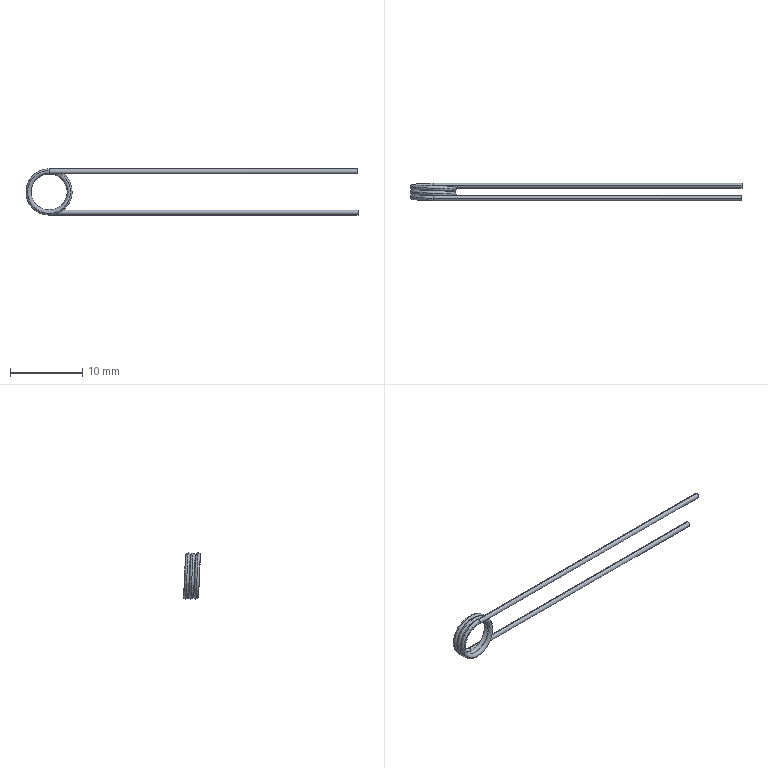Part | SolidWorks | features CompositeCurve 1, Helix 1, MoveFace 1, Sweep 1 | 1 solid | 9 faces | box 46.05 x 2.45 x 6.4 mm | volume 49.652 mm3 | cylinder 4 | spline 3 | plane 2 | commonest cylinder face diameters 0.7 x4
STEP:
#1=CARTESIAN_POINT('',(42.85,1.75,-3.2));
#2=VERTEX_POINT('',#1);
#3=CARTESIAN_POINT('',(42.85,1.75,-2.5));
#4=VERTEX_POINT('',#3);
#5=CARTESIAN_POINT('',(42.85,1.75,-2.85));
#6=DIRECTION('',(1.,0.,0.));
#7=DIRECTION('',(0.,0.00009155,-1.));
#8=AXIS2_PLACEMENT_3D('',#5,#6,#7);
#9=CIRCLE('',#8,0.35);
#10=EDGE_CURVE('',#2,#4,#9,.T.);
#11=ORIENTED_EDGE('',*,*,#10,.F.);
#12=CARTESIAN_POINT('',(-0.000000536,1.75,-3.2));
#13=VERTEX_POINT('',#12);
#14=CARTESIAN_POINT('',(12.85,1.75,-3.2));
#15=DIRECTION('',(-1.,0.,0.));
#16=VECTOR('',#15,1000.);
#17=LINE('',#14,#16);
#18=EDGE_CURVE('',#2,#13,#17,.T.);
#19=ORIENTED_EDGE('',*,*,#18,.T.);
#20=CARTESIAN_POINT('',(-0.006305,2.074,-2.979));
#21=VERTEX_POINT('',#20);
#22=CARTESIAN_POINT('',(0.,1.75,-2.85));
#23=DIRECTION('',(1.,0.,0.));
#24=DIRECTION('',(0.,0.00009155,-1.));
#25=AXIS2_PLACEMENT_3D('',#22,#23,#24);
#26=CIRCLE('',#25,0.35);
#27=EDGE_CURVE('',#13,#21,#26,.T.);
#28=ORIENTED_EDGE('',*,*,#27,.T.);
#29=CARTESIAN_POINT('',(0.,1.75,-2.5));
#30=VERTEX_POINT('',#29);
#31=CARTESIAN_POINT('',(0.,1.75,-2.85));
#32=DIRECTION('',(1.,0.,0.));
#33=DIRECTION('',(0.,0.00009155,-1.));
#34=AXIS2_PLACEMENT_3D('',#31,#32,#33);
#35=CIRCLE('',#34,0.35);
#36=EDGE_CURVE('',#21,#30,#35,.T.);
#37=ORIENTED_EDGE('',*,*,#36,.T.);
#38=CARTESIAN_POINT('',(12.85,1.75,-2.5));
#39=DIRECTION('',(-1.,0.,0.));
#40=VECTOR('',#39,1000.);
#41=LINE('',#38,#40);
#42=EDGE_CURVE('',#4,#30,#41,.T.);
#43=ORIENTED_EDGE('',*,*,#42,.F.);
#44=EDGE_LOOP('',(#11,#19,#28,#37,#43));
#45=FACE_OUTER_BOUND('',#44,.T.);
#46=CARTESIAN_POINT('',(12.85,1.75,-2.85));
#47=DIRECTION('',(-1.,0.,0.));
#48=DIRECTION('',(0.,0.,1.));
#49=AXIS2_PLACEMENT_3D('',#46,#47,#48);
#50=CYLINDRICAL_SURFACE('',#49,0.35);
#51=ADVANCED_FACE('',(#45),#50,.T.);
#52=CARTESIAN_POINT('',(0.006305,0.3239,2.979));
#53=VERTEX_POINT('',#52);
#54=CARTESIAN_POINT('',(0.,0.,3.2));
#55=VERTEX_POINT('',#54);
#56=CARTESIAN_POINT('',(0.006305,0.3239,2.979));
#57=CARTESIAN_POINT('',(0.01048,0.2681,3.104));
#58=CARTESIAN_POINT('',(0.005425,0.1388,3.2));
#59=CARTESIAN_POINT('',(0.,0.,3.2));
#60=B_SPLINE_CURVE_WITH_KNOTS('',3,(#56,#57,#58,#59),.UNSPECIFIED.,.F.,.F.,(4,4),(0.00002721,0.1895),.UNSPECIFIED.);
#61=EDGE_CURVE('',#53,#55,#60,.T.);
#62=ORIENTED_EDGE('',*,*,#61,.T.);
#63=CARTESIAN_POINT('',(42.85,0.,3.2));
#64=VERTEX_POINT('',#63);
#65=CARTESIAN_POINT('',(0.,0.,3.2));
#66=DIRECTION('',(1.,0.,0.));
#67=VECTOR('',#66,1000.);
#68=LINE('',#65,#67);
#69=EDGE_CURVE('',#55,#64,#68,.T.);
#70=ORIENTED_EDGE('',*,*,#69,.T.);
#71=CARTESIAN_POINT('',(42.85,0.,2.5));
#72=VERTEX_POINT('',#71);
#73=CARTESIAN_POINT('',(42.85,0.,2.85));
#74=DIRECTION('',(-1.,0.,0.));
#75=DIRECTION('',(0.,0.,1.));
#76=AXIS2_PLACEMENT_3D('',#73,#74,#75);
#77=CIRCLE('',#76,0.35);
#78=EDGE_CURVE('',#64,#72,#77,.T.);
#79=ORIENTED_EDGE('',*,*,#78,.T.);
#80=CARTESIAN_POINT('',(0.,0.,2.5));
#81=VERTEX_POINT('',#80);
#82=CARTESIAN_POINT('',(0.,0.,2.5));
#83=DIRECTION('',(1.,0.,0.));
#84=VECTOR('',#83,1000.);
#85=LINE('',#82,#84);
#86=EDGE_CURVE('',#81,#72,#85,.T.);
#87=ORIENTED_EDGE('',*,*,#86,.F.);
#88=CARTESIAN_POINT('',(0.,0.,2.85));
#89=DIRECTION('',(-1.,0.,0.));
#90=DIRECTION('',(0.,0.,1.));
#91=AXIS2_PLACEMENT_3D('',#88,#89,#90);
#92=CIRCLE('',#91,0.35);
#93=EDGE_CURVE('',#53,#81,#92,.T.);
#94=ORIENTED_EDGE('',*,*,#93,.F.);
#95=EDGE_LOOP('',(#62,#70,#79,#87,#94));
#96=FACE_OUTER_BOUND('',#95,.T.);
#97=CARTESIAN_POINT('',(0.,0.,2.85));
#98=DIRECTION('',(1.,0.,0.));
#99=DIRECTION('',(0.,0.,-1.));
#100=AXIS2_PLACEMENT_3D('',#97,#98,#99);
#101=CYLINDRICAL_SURFACE('',#100,0.35);
#102=ADVANCED_FACE('',(#96),#101,.T.);
#103=ORIENTED_EDGE('',*,*,#18,.F.);
#104=CARTESIAN_POINT('',(42.85,1.75,-2.85));
#105=DIRECTION('',(1.,0.,0.));
#106=DIRECTION('',(0.,0.00009155,-1.));
#107=AXIS2_PLACEMENT_3D('',#104,#105,#106);
#108=CIRCLE('',#107,0.35);
#109=EDGE_CURVE('',#4,#2,#108,.T.);
#110=ORIENTED_EDGE('',*,*,#109,.F.);
#111=ORIENTED_EDGE('',*,*,#42,.T.);
#112=CARTESIAN_POINT('',(0.006304,1.426,-2.979));
#113=VERTEX_POINT('',#112);
#114=CARTESIAN_POINT('',(0.,1.75,-2.85));
#115=DIRECTION('',(1.,0.,0.));
#116=DIRECTION('',(0.,0.00009155,-1.));
#117=AXIS2_PLACEMENT_3D('',#114,#115,#116);
#118=CIRCLE('',#117,0.35);
#119=EDGE_CURVE('',#30,#113,#118,.T.);
#120=ORIENTED_EDGE('',*,*,#119,.T.);
#121=CARTESIAN_POINT('',(0.,1.75,-2.85));
#122=DIRECTION('',(1.,0.,0.));
#123=DIRECTION('',(0.,0.00009155,-1.));
#124=AXIS2_PLACEMENT_3D('',#121,#122,#123);
#125=CIRCLE('',#124,0.35);
#126=EDGE_CURVE('',#113,#13,#125,.T.);
#127=ORIENTED_EDGE('',*,*,#126,.T.);
#128=EDGE_LOOP('',(#103,#110,#111,#120,#127));
#129=FACE_OUTER_BOUND('',#128,.T.);
#130=CARTESIAN_POINT('',(12.85,1.75,-2.85));
#131=DIRECTION('',(-1.,0.,0.));
#132=DIRECTION('',(0.,0.,1.));
#133=AXIS2_PLACEMENT_3D('',#130,#131,#132);
#134=CYLINDRICAL_SURFACE('',#133,0.35);
#135=ADVANCED_FACE('',(#129),#134,.T.);
#136=ORIENTED_EDGE('',*,*,#36,.F.);
#137=CARTESIAN_POINT('',(0.006305,0.3239,2.979));
#138=CARTESIAN_POINT('',(-0.7712,0.3519,2.981));
#139=CARTESIAN_POINT('',(-1.545,0.381,2.663));
#140=CARTESIAN_POINT('',(-2.649,0.4392,1.566));
#141=CARTESIAN_POINT('',(-2.975,0.4683,0.7939));
#142=CARTESIAN_POINT('',(-2.98,0.5195,-0.5733));
#143=CARTESIAN_POINT('',(-2.806,0.5413,-1.156));
#144=CARTESIAN_POINT('',(-2.162,0.585,-2.13));
#145=CARTESIAN_POINT('',(-1.69,0.6069,-2.521));
#146=CARTESIAN_POINT('',(-0.4324,0.658,-3.048));
#147=CARTESIAN_POINT('',(0.405,0.6871,-3.052));
#148=CARTESIAN_POINT('',(1.67,0.7383,-2.534));
#149=CARTESIAN_POINT('',(2.142,0.7601,-2.15));
#150=CARTESIAN_POINT('',(2.795,0.8037,-1.182));
#151=CARTESIAN_POINT('',(2.976,0.8257,-0.5972));
#152=CARTESIAN_POINT('',(2.981,0.8768,0.7668));
#153=CARTESIAN_POINT('',(2.665,0.9058,1.542));
#154=CARTESIAN_POINT('',(1.702,0.957,2.513));
#155=CARTESIAN_POINT('',(1.167,0.9788,2.801));
#156=CARTESIAN_POINT('',(0.02248,1.022,3.035));
#157=CARTESIAN_POINT('',(-0.587,1.044,2.978));
#158=CARTESIAN_POINT('',(-1.849,1.096,2.461));
#159=CARTESIAN_POINT('',(-2.445,1.125,1.872));
#160=CARTESIAN_POINT('',(-2.973,1.176,0.6109));
#161=CARTESIAN_POINT('',(-3.035,1.198,0.005944));
#162=CARTESIAN_POINT('',(-2.812,1.241,-1.14));
#163=CARTESIAN_POINT('',(-2.526,1.263,-1.682));
#164=CARTESIAN_POINT('',(-1.566,1.314,-2.65));
#165=CARTESIAN_POINT('',(-0.7938,1.343,-2.975));
#166=CARTESIAN_POINT('',(0.5733,1.395,-2.98));
#167=CARTESIAN_POINT('',(1.156,1.416,-2.806));
#168=CARTESIAN_POINT('',(2.13,1.46,-2.162));
#169=CARTESIAN_POINT('',(2.521,1.482,-1.69));
#170=CARTESIAN_POINT('',(3.048,1.533,-0.4324));
#171=CARTESIAN_POINT('',(3.052,1.562,0.405));
#172=CARTESIAN_POINT('',(2.534,1.613,1.67));
#173=CARTESIAN_POINT('',(2.15,1.635,2.142));
#174=CARTESIAN_POINT('',(1.182,1.679,2.795));
#175=CARTESIAN_POINT('',(0.5972,1.701,2.976));
#176=CARTESIAN_POINT('',(-0.7668,1.752,2.981));
#177=CARTESIAN_POINT('',(-1.542,1.781,2.665));
#178=CARTESIAN_POINT('',(-2.513,1.832,1.702));
#179=CARTESIAN_POINT('',(-2.801,1.854,1.167));
#180=CARTESIAN_POINT('',(-3.034,1.897,0.0225));
#181=CARTESIAN_POINT('',(-2.978,1.919,-0.587));
#182=CARTESIAN_POINT('',(-2.46,1.971,-1.85));
#183=CARTESIAN_POINT('',(-1.872,2.,-2.445));
#184=CARTESIAN_POINT('',(-0.7917,2.043,-2.897));
#185=CARTESIAN_POINT('',(-0.4042,2.058,-2.976));
#186=CARTESIAN_POINT('',(-0.006305,2.074,-2.979));
#187=B_SPLINE_CURVE_WITH_KNOTS('',3,(#137,#138,#139,#140,#141,#142,#143,#144,#145,#146,#147,#148,#149,#150,#151,#152,#153,#154,#155,#156,#157,#158,#159,#160,#161,#162,#163,#164,#165,#166,#167,#168,#169,#170,#171,#172,#173,#174,#175,#176,#177,#178,#179,#180,#181,#182,#183,#184,#185,#186),.UNSPECIFIED.,.F.,.F.,(4,2,2,2,2,2,2,2,2,2,2,2,2,2,2,2,2,2,2,2,2,2,2,2,4),(0.,0.04998,0.09999,0.1375,0.175,0.225,0.2625,0.3,0.35,0.3875,0.425,0.475,0.5125,0.55,0.6,0.6375,0.675,0.725,0.7625,0.8,0.85,0.8875,0.925,0.975,1.),.UNSPECIFIED.);
#188=EDGE_CURVE('',#53,#21,#187,.T.);
#189=ORIENTED_EDGE('',*,*,#188,.F.);
#190=ORIENTED_EDGE('',*,*,#93,.T.);
#191=CARTESIAN_POINT('',(-0.006304,-0.3239,2.979));
#192=VERTEX_POINT('',#191);
#193=CARTESIAN_POINT('',(0.,0.,2.85));
#194=DIRECTION('',(-1.,0.,0.));
#195=DIRECTION('',(0.,0.,1.));
#196=AXIS2_PLACEMENT_3D('',#193,#194,#195);
#197=CIRCLE('',#196,0.35);
#198=EDGE_CURVE('',#81,#192,#197,.T.);
#199=ORIENTED_EDGE('',*,*,#198,.T.);
#200=CARTESIAN_POINT('',(0.006304,1.426,-2.979));
#201=CARTESIAN_POINT('',(-0.379,1.413,-2.98));
#202=CARTESIAN_POINT('',(-0.7673,1.398,-2.904));
#203=CARTESIAN_POINT('',(-1.851,1.354,-2.461));
#204=CARTESIAN_POINT('',(-2.445,1.325,-1.871));
#205=CARTESIAN_POINT('',(-2.973,1.274,-0.6122));
#206=CARTESIAN_POINT('',(-3.035,1.252,-0.003211));
#207=CARTESIAN_POINT('',(-2.811,1.209,1.143));
#208=CARTESIAN_POINT('',(-2.527,1.187,1.681));
#209=CARTESIAN_POINT('',(-1.565,1.136,2.652));
#210=CARTESIAN_POINT('',(-0.792,1.107,2.975));
#211=CARTESIAN_POINT('',(0.572,1.056,2.981));
#212=CARTESIAN_POINT('',(1.158,1.034,2.805));
#213=CARTESIAN_POINT('',(2.132,0.99,2.16));
#214=CARTESIAN_POINT('',(2.52,0.9682,1.692));
#215=CARTESIAN_POINT('',(3.049,0.917,0.4308));
#216=CARTESIAN_POINT('',(3.052,0.8879,-0.4067));
#217=CARTESIAN_POINT('',(2.535,0.8368,-1.669));
#218=CARTESIAN_POINT('',(2.148,0.8149,-2.144));
#219=CARTESIAN_POINT('',(1.18,0.7712,-2.796));
#220=CARTESIAN_POINT('',(0.5985,0.7494,-2.976));
#221=CARTESIAN_POINT('',(-0.7686,0.6982,-2.981));
#222=CARTESIAN_POINT('',(-1.544,0.6692,-2.664));
#223=CARTESIAN_POINT('',(-2.512,0.6181,-1.703));
#224=CARTESIAN_POINT('',(-2.802,0.5961,-1.164));
#225=CARTESIAN_POINT('',(-3.035,0.5525,-0.01977));
#226=CARTESIAN_POINT('',(-2.978,0.5307,0.5858));
#227=CARTESIAN_POINT('',(-2.46,0.4795,1.851));
#228=CARTESIAN_POINT('',(-1.87,0.4504,2.445));
#229=CARTESIAN_POINT('',(-0.6122,0.3993,2.973));
#230=CARTESIAN_POINT('',(-0.003226,0.3774,3.035));
#231=CARTESIAN_POINT('',(1.143,0.3337,2.811));
#232=CARTESIAN_POINT('',(1.681,0.3119,2.527));
#233=CARTESIAN_POINT('',(2.652,0.2607,1.565));
#234=CARTESIAN_POINT('',(2.975,0.2317,0.792));
#235=CARTESIAN_POINT('',(2.981,0.1806,-0.572));
#236=CARTESIAN_POINT('',(2.805,0.1586,-1.158));
#237=CARTESIAN_POINT('',(2.16,0.115,-2.132));
#238=CARTESIAN_POINT('',(1.692,0.09317,-2.52));
#239=CARTESIAN_POINT('',(0.4308,0.04196,-3.049));
#240=CARTESIAN_POINT('',(-0.4067,0.01292,-3.052));
#241=CARTESIAN_POINT('',(-1.669,-0.03818,-2.535));
#242=CARTESIAN_POINT('',(-2.144,-0.06013,-2.148));
#243=CARTESIAN_POINT('',(-2.796,-0.1038,-1.18));
#244=CARTESIAN_POINT('',(-2.976,-0.1256,-0.5985));
#245=CARTESIAN_POINT('',(-2.981,-0.1768,0.7687));
#246=CARTESIAN_POINT('',(-2.663,-0.2059,1.544));
#247=CARTESIAN_POINT('',(-1.567,-0.2642,2.65));
#248=CARTESIAN_POINT('',(-0.7966,-0.2932,2.975));
#249=CARTESIAN_POINT('',(-0.006304,-0.3239,2.979));
#250=B_SPLINE_CURVE_WITH_KNOTS('',3,(#200,#201,#202,#203,#204,#205,#206,#207,#208,#209,#210,#211,#212,#213,#214,#215,#216,#217,#218,#219,#220,#221,#222,#223,#224,#225,#226,#227,#228,#229,#230,#231,#232,#233,#234,#235,#236,#237,#238,#239,#240,#241,#242,#243,#244,#245,#246,#247,#248,#249),.UNSPECIFIED.,.F.,.F.,(4,2,2,2,2,2,2,2,2,2,2,2,2,2,2,2,2,2,2,2,2,2,2,2,4),(0.,0.02496,0.07501,0.1125,0.15,0.2,0.2375,0.275,0.325,0.3625,0.4,0.45,0.4875,0.525,0.575,0.6125,0.65,0.7,0.7375,0.775,0.825,0.8625,0.9,0.95,1.),.UNSPECIFIED.);
#251=EDGE_CURVE('',#113,#192,#250,.T.);
#252=ORIENTED_EDGE('',*,*,#251,.F.);
#253=ORIENTED_EDGE('',*,*,#119,.F.);
#254=EDGE_LOOP('',(#136,#189,#190,#199,#252,#253));
#255=FACE_OUTER_BOUND('',#254,.T.);
#256=CARTESIAN_POINT('',(-0.01261,2.073,-2.978));
#257=CARTESIAN_POINT('',(-0.9931,2.036,-2.974));
#258=CARTESIAN_POINT('',(-1.942,2.,-2.452));
#259=CARTESIAN_POINT('',(-3.022,1.927,-0.8338));
#260=CARTESIAN_POINT('',(-3.123,1.89,0.2539));
#261=CARTESIAN_POINT('',(-2.369,1.817,2.048));
#262=CARTESIAN_POINT('',(-1.523,1.781,2.732));
#263=CARTESIAN_POINT('',(0.3864,1.708,3.111));
#264=CARTESIAN_POINT('',(1.43,1.671,2.788));
#265=CARTESIAN_POINT('',(2.798,1.599,1.405));
#266=CARTESIAN_POINT('',(3.107,1.562,0.3615));
#267=CARTESIAN_POINT('',(2.726,1.489,-1.547));
#268=CARTESIAN_POINT('',(2.029,1.453,-2.388));
#269=CARTESIAN_POINT('',(0.2273,1.38,-3.123));
#270=CARTESIAN_POINT('',(-0.8551,1.343,-3.009));
#271=CARTESIAN_POINT('',(-2.473,1.271,-1.927));
#272=CARTESIAN_POINT('',(-2.982,1.234,-0.9604));
#273=CARTESIAN_POINT('',(-2.972,1.161,0.9852));
#274=CARTESIAN_POINT('',(-2.453,1.125,1.942));
#275=CARTESIAN_POINT('',(-0.8335,1.052,3.022));
#276=CARTESIAN_POINT('',(0.2539,1.015,3.123));
#277=CARTESIAN_POINT('',(2.048,0.9425,2.369));
#278=CARTESIAN_POINT('',(2.732,0.9059,1.523));
#279=CARTESIAN_POINT('',(3.111,0.8331,-0.3864));
#280=CARTESIAN_POINT('',(2.788,0.7965,-1.43));
#281=CARTESIAN_POINT('',(1.405,0.7237,-2.798));
#282=CARTESIAN_POINT('',(0.3615,0.6872,-3.107));
#283=CARTESIAN_POINT('',(-1.547,0.6143,-2.726));
#284=CARTESIAN_POINT('',(-2.388,0.5777,-2.029));
#285=CARTESIAN_POINT('',(-3.123,0.505,-0.2273));
#286=CARTESIAN_POINT('',(-3.009,0.4684,0.8554));
#287=CARTESIAN_POINT('',(-1.927,0.3956,2.473));
#288=CARTESIAN_POINT('',(-0.9676,0.3593,2.982));
#289=CARTESIAN_POINT('',(0.01261,0.3226,2.978));
#290=CARTESIAN_POINT('',(-0.0161,2.162,-2.771));
#291=CARTESIAN_POINT('',(-0.9269,2.125,-2.766));
#292=CARTESIAN_POINT('',(-1.811,2.089,-2.279));
#293=CARTESIAN_POINT('',(-2.813,2.016,-0.7712));
#294=CARTESIAN_POINT('',(-2.906,1.979,0.2409));
#295=CARTESIAN_POINT('',(-2.201,1.907,1.909));
#296=CARTESIAN_POINT('',(-1.413,1.87,2.545));
#297=CARTESIAN_POINT('',(0.3644,1.797,2.894));
#298=CARTESIAN_POINT('',(1.334,1.761,2.592));
#299=CARTESIAN_POINT('',(2.606,1.688,1.303));
#300=CARTESIAN_POINT('',(2.892,1.651,0.3318));
#301=CARTESIAN_POINT('',(2.535,1.579,-1.444));
#302=CARTESIAN_POINT('',(1.884,1.542,-2.225));
#303=CARTESIAN_POINT('',(0.2064,1.469,-2.907));
#304=CARTESIAN_POINT('',(-0.8001,1.433,-2.799));
#305=CARTESIAN_POINT('',(-2.304,1.36,-1.789));
#306=CARTESIAN_POINT('',(-2.777,1.323,-0.8894));
#307=CARTESIAN_POINT('',(-2.764,1.25,0.9216));
#308=CARTESIAN_POINT('',(-2.279,1.214,1.81));
#309=CARTESIAN_POINT('',(-0.771,1.141,2.814));
#310=CARTESIAN_POINT('',(0.2409,1.104,2.906));
#311=CARTESIAN_POINT('',(1.909,1.032,2.201));
#312=CARTESIAN_POINT('',(2.545,0.9951,1.413));
#313=CARTESIAN_POINT('',(2.894,0.9223,-0.3644));
#314=CARTESIAN_POINT('',(2.592,0.8857,-1.334));
#315=CARTESIAN_POINT('',(1.303,0.8129,-2.606));
#316=CARTESIAN_POINT('',(0.3318,0.7764,-2.892));
#317=CARTESIAN_POINT('',(-1.444,0.7035,-2.535));
#318=CARTESIAN_POINT('',(-2.225,0.667,-1.884));
#319=CARTESIAN_POINT('',(-2.907,0.5942,-0.2064));
#320=CARTESIAN_POINT('',(-2.798,0.5576,0.8003));
#321=CARTESIAN_POINT('',(-1.789,0.4848,2.304));
#322=CARTESIAN_POINT('',(-0.8958,0.4485,2.776));
#323=CARTESIAN_POINT('',(0.0161,0.4118,2.771));
#324=CARTESIAN_POINT('',(-0.008888,1.977,-2.5));
#325=CARTESIAN_POINT('',(-0.8283,1.941,-2.497));
#326=CARTESIAN_POINT('',(-1.629,1.904,-2.059));
#327=CARTESIAN_POINT('',(-2.536,1.832,-0.7012));
#328=CARTESIAN_POINT('',(-2.622,1.795,0.2114));
#329=CARTESIAN_POINT('',(-1.989,1.722,1.718));
#330=CARTESIAN_POINT('',(-1.28,1.686,2.292));
#331=CARTESIAN_POINT('',(0.3232,1.613,2.612));
#332=CARTESIAN_POINT('',(1.199,1.576,2.341));
#333=CARTESIAN_POINT('',(2.349,1.503,1.18));
#334=CARTESIAN_POINT('',(2.608,1.467,0.3051));
#335=CARTESIAN_POINT('',(2.29,1.394,-1.298));
#336=CARTESIAN_POINT('',(1.704,1.358,-2.003));
#337=CARTESIAN_POINT('',(0.1914,1.285,-2.622));
#338=CARTESIAN_POINT('',(-0.716,1.248,-2.526));
#339=CARTESIAN_POINT('',(-2.075,1.175,-1.618));
#340=CARTESIAN_POINT('',(-2.503,1.139,-0.808));
#341=CARTESIAN_POINT('',(-2.495,1.066,0.8264));
#342=CARTESIAN_POINT('',(-2.06,1.029,1.628));
#343=CARTESIAN_POINT('',(-0.701,0.9565,2.537));
#344=CARTESIAN_POINT('',(0.2114,0.92,2.622));
#345=CARTESIAN_POINT('',(1.718,0.8471,1.989));
#346=CARTESIAN_POINT('',(2.292,0.8107,1.28));
#347=CARTESIAN_POINT('',(2.612,0.7378,-0.3232));
#348=CARTESIAN_POINT('',(2.341,0.7013,-1.199));
#349=CARTESIAN_POINT('',(1.18,0.6284,-2.349));
#350=CARTESIAN_POINT('',(0.3051,0.5919,-2.608));
#351=CARTESIAN_POINT('',(-1.298,0.519,-2.29));
#352=CARTESIAN_POINT('',(-2.003,0.4825,-1.704));
#353=CARTESIAN_POINT('',(-2.622,0.4096,-0.1914));
#354=CARTESIAN_POINT('',(-2.525,0.3732,0.7162));
#355=CARTESIAN_POINT('',(-1.619,0.3003,2.075));
#356=CARTESIAN_POINT('',(-0.8134,0.2639,2.503));
#357=CARTESIAN_POINT('',(0.008889,0.2274,2.5));
#358=CARTESIAN_POINT('',(0.008895,1.522,-2.5));
#359=CARTESIAN_POINT('',(-0.8105,1.486,-2.503));
#360=CARTESIAN_POINT('',(-1.614,1.45,-2.071));
#361=CARTESIAN_POINT('',(-2.532,1.377,-0.7193));
#362=CARTESIAN_POINT('',(-2.623,1.34,0.1927));
#363=CARTESIAN_POINT('',(-2.001,1.267,1.704));
#364=CARTESIAN_POINT('',(-1.296,1.231,2.283));
#365=CARTESIAN_POINT('',(0.3046,1.158,2.614));
#366=CARTESIAN_POINT('',(1.182,1.121,2.35));
#367=CARTESIAN_POINT('',(2.341,1.048,1.197));
#368=CARTESIAN_POINT('',(2.606,1.012,0.3236));
#369=CARTESIAN_POINT('',(2.299,0.9391,-1.282));
#370=CARTESIAN_POINT('',(1.719,0.9026,-1.991));
#371=CARTESIAN_POINT('',(0.2101,0.8297,-2.62));
#372=CARTESIAN_POINT('',(-0.6981,0.7933,-2.531));
#373=CARTESIAN_POINT('',(-2.064,0.7204,-1.633));
#374=CARTESIAN_POINT('',(-2.497,0.6839,-0.8259));
#375=CARTESIAN_POINT('',(-2.501,0.611,0.8087));
#376=CARTESIAN_POINT('',(-2.071,0.5745,1.614));
#377=CARTESIAN_POINT('',(-0.7191,0.5016,2.532));
#378=CARTESIAN_POINT('',(0.1927,0.4651,2.623));
#379=CARTESIAN_POINT('',(1.704,0.3922,2.001));
#380=CARTESIAN_POINT('',(2.283,0.3558,1.296));
#381=CARTESIAN_POINT('',(2.614,0.2829,-0.3046));
#382=CARTESIAN_POINT('',(2.35,0.2464,-1.182));
#383=CARTESIAN_POINT('',(1.197,0.1735,-2.341));
#384=CARTESIAN_POINT('',(0.3236,0.137,-2.606));
#385=CARTESIAN_POINT('',(-1.282,0.0641,-2.299));
#386=CARTESIAN_POINT('',(-1.991,0.02763,-1.719));
#387=CARTESIAN_POINT('',(-2.62,-0.04528,-0.2101));
#388=CARTESIAN_POINT('',(-2.531,-0.08173,0.6983));
#389=CARTESIAN_POINT('',(-1.633,-0.1546,2.064));
#390=CARTESIAN_POINT('',(-0.8313,-0.191,2.497));
#391=CARTESIAN_POINT('',(-0.008894,-0.2275,2.5));
#392=CARTESIAN_POINT('',(0.0161,1.338,-2.771));
#393=CARTESIAN_POINT('',(-0.8947,1.302,-2.777));
#394=CARTESIAN_POINT('',(-1.785,1.265,-2.3));
#395=CARTESIAN_POINT('',(-2.804,1.192,-0.804));
#396=CARTESIAN_POINT('',(-2.908,1.156,0.2071));
#397=CARTESIAN_POINT('',(-2.223,1.083,1.884));
#398=CARTESIAN_POINT('',(-1.443,1.046,2.528));
#399=CARTESIAN_POINT('',(0.3307,0.9736,2.899));
#400=CARTESIAN_POINT('',(1.304,0.937,2.608));
#401=CARTESIAN_POINT('',(2.591,0.8642,1.333));
#402=CARTESIAN_POINT('',(2.888,0.8277,0.3653));
#403=CARTESIAN_POINT('',(2.552,0.7548,-1.415));
#404=CARTESIAN_POINT('',(1.91,0.7183,-2.203));
#405=CARTESIAN_POINT('',(0.2402,0.6455,-2.904));
#406=CARTESIAN_POINT('',(-0.7677,0.6089,-2.808));
#407=CARTESIAN_POINT('',(-2.284,0.5361,-1.816));
#408=CARTESIAN_POINT('',(-2.766,0.4995,-0.9217));
#409=CARTESIAN_POINT('',(-2.775,0.4267,0.8895));
#410=CARTESIAN_POINT('',(-2.3,0.3902,1.784));
#411=CARTESIAN_POINT('',(-0.8038,0.3173,2.805));
#412=CARTESIAN_POINT('',(0.2071,0.2808,2.908));
#413=CARTESIAN_POINT('',(1.884,0.208,2.223));
#414=CARTESIAN_POINT('',(2.528,0.1714,1.443));
#415=CARTESIAN_POINT('',(2.899,0.09857,-0.3307));
#416=CARTESIAN_POINT('',(2.608,0.06204,-1.304));
#417=CARTESIAN_POINT('',(1.333,-0.01079,-2.591));
#418=CARTESIAN_POINT('',(0.3653,-0.0473,-2.888));
#419=CARTESIAN_POINT('',(-1.415,-0.1202,-2.552));
#420=CARTESIAN_POINT('',(-2.203,-0.1567,-1.91));
#421=CARTESIAN_POINT('',(-2.904,-0.2295,-0.2402));
#422=CARTESIAN_POINT('',(-2.807,-0.2661,0.7679));
#423=CARTESIAN_POINT('',(-1.816,-0.3389,2.283));
#424=CARTESIAN_POINT('',(-0.9282,-0.3752,2.766));
#425=CARTESIAN_POINT('',(-0.0161,-0.4119,2.771));
#426=CARTESIAN_POINT('',(0.01261,1.427,-2.978));
#427=CARTESIAN_POINT('',(-0.9679,1.391,-2.982));
#428=CARTESIAN_POINT('',(-1.922,1.354,-2.469));
#429=CARTESIAN_POINT('',(-3.015,1.282,-0.8595));
#430=CARTESIAN_POINT('',(-3.125,1.245,0.2275));
#431=CARTESIAN_POINT('',(-2.386,1.172,2.028));
#432=CARTESIAN_POINT('',(-1.546,1.136,2.72));
#433=CARTESIAN_POINT('',(0.36,1.063,3.114));
#434=CARTESIAN_POINT('',(1.406,1.026,2.8));
#435=CARTESIAN_POINT('',(2.787,0.9536,1.429));
#436=CARTESIAN_POINT('',(3.104,0.917,0.3878));
#437=CARTESIAN_POINT('',(2.739,0.8442,-1.524));
#438=CARTESIAN_POINT('',(2.049,0.8076,-2.37));
#439=CARTESIAN_POINT('',(0.2537,0.7349,-3.121));
#440=CARTESIAN_POINT('',(-0.8297,0.6983,-3.016));
#441=CARTESIAN_POINT('',(-2.457,0.6254,-1.948));
#442=CARTESIAN_POINT('',(-2.974,0.5889,-0.9857));
#443=CARTESIAN_POINT('',(-2.981,0.5161,0.96));
#444=CARTESIAN_POINT('',(-2.469,0.4795,1.921));
#445=CARTESIAN_POINT('',(-0.8592,0.4067,3.015));
#446=CARTESIAN_POINT('',(0.2275,0.3701,3.125));
#447=CARTESIAN_POINT('',(2.028,0.2974,2.386));
#448=CARTESIAN_POINT('',(2.72,0.2608,1.546));
#449=CARTESIAN_POINT('',(3.114,0.1879,-0.36));
#450=CARTESIAN_POINT('',(2.8,0.1514,-1.406));
#451=CARTESIAN_POINT('',(1.429,0.07861,-2.787));
#452=CARTESIAN_POINT('',(0.3878,0.04204,-3.104));
#453=CARTESIAN_POINT('',(-1.524,-0.03081,-2.739));
#454=CARTESIAN_POINT('',(-2.371,-0.06738,-2.049));
#455=CARTESIAN_POINT('',(-3.121,-0.1401,-0.2537));
#456=CARTESIAN_POINT('',(-3.016,-0.1767,0.83));
#457=CARTESIAN_POINT('',(-1.948,-0.2496,2.456));
#458=CARTESIAN_POINT('',(-0.993,-0.2858,2.974));
#459=CARTESIAN_POINT('',(-0.01261,-0.3225,2.978));
#460=B_SPLINE_SURFACE_WITH_KNOTS('',3,3,((#256,#257,#258,#259,#260,#261,#262,#263,#264,#265,#266,#267,#268,#269,#270,#271,#272,#273,#274,#275,#276,#277,#278,#279,#280,#281,#282,#283,#284,#285,#286,#287,#288,#289),(#290,#291,#292,#293,#294,#295,#296,#297,#298,#299,#300,#301,#302,#303,#304,#305,#306,#307,#308,#309,#310,#311,#312,#313,#314,#315,#316,#317,#318,#319,#320,#321,#322,#323),(#324,#325,#326,#327,#328,#329,#330,#331,#332,#333,#334,#335,#336,#337,#338,#339,#340,#341,#342,#343,#344,#345,#346,#347,#348,#349,#350,#351,#352,#353,#354,#355,#356,#357),(#358,#359,#360,#361,#362,#363,#364,#365,#366,#367,#368,#369,#370,#371,#372,#373,#374,#375,#376,#377,#378,#379,#380,#381,#382,#383,#384,#385,#386,#387,#388,#389,#390,#391),(#392,#393,#394,#395,#396,#397,#398,#399,#400,#401,#402,#403,#404,#405,#406,#407,#408,#409,#410,#411,#412,#413,#414,#415,#416,#417,#418,#419,#420,#421,#422,#423,#424,#425),(#426,#427,#428,#429,#430,#431,#432,#433,#434,#435,#436,#437,#438,#439,#440,#441,#442,#443,#444,#445,#446,#447,#448,#449,#450,#451,#452,#453,#454,#455,#456,#457,#458,#459)),.UNSPECIFIED.,.F.,.F.,.F.,(4,2,4),(4,2,2,2,2,2,2,2,2,2,2,2,2,2,2,2,4),(0.1895,0.5,0.8106),(0.,0.0625,0.125,0.1875,0.25,0.3125,0.375,0.4375,0.5,0.5625,0.625,0.6875,0.75,0.8125,0.875,0.9375,1.),.UNSPECIFIED.);
#461=ADVANCED_FACE('',(#255),#460,.F.);
#462=ORIENTED_EDGE('',*,*,#126,.F.);
#463=ORIENTED_EDGE('',*,*,#251,.T.);
#464=CARTESIAN_POINT('',(0.,0.,3.2));
#465=CARTESIAN_POINT('',(-0.005423,-0.1387,3.2));
#466=CARTESIAN_POINT('',(-0.01048,-0.268,3.104));
#467=CARTESIAN_POINT('',(-0.006304,-0.3239,2.979));
#468=B_SPLINE_CURVE_WITH_KNOTS('',3,(#464,#465,#466,#467),.UNSPECIFIED.,.F.,.F.,(4,4),(0.8106,1.),.UNSPECIFIED.);
#469=EDGE_CURVE('',#55,#192,#468,.T.);
#470=ORIENTED_EDGE('',*,*,#469,.F.);
#471=CARTESIAN_POINT('',(-0.000000536,1.75,-3.2));
#472=CARTESIAN_POINT('',(-0.4215,1.735,-3.2));
#473=CARTESIAN_POINT('',(-0.8371,1.721,-3.117));
#474=CARTESIAN_POINT('',(-2.001,1.677,-2.635));
#475=CARTESIAN_POINT('',(-2.635,1.648,-2.));
#476=CARTESIAN_POINT('',(-3.197,1.597,-0.6438));
#477=CARTESIAN_POINT('',(-3.261,1.575,0.01064));
#478=CARTESIAN_POINT('',(-3.015,1.531,1.241));
#479=CARTESIAN_POINT('',(-2.708,1.51,1.817));
#480=CARTESIAN_POINT('',(-1.669,1.458,2.857));
#481=CARTESIAN_POINT('',(-0.8382,1.429,3.2));
#482=CARTESIAN_POINT('',(0.6287,1.378,3.2));
#483=CARTESIAN_POINT('',(1.258,1.356,3.008));
#484=CARTESIAN_POINT('',(2.3,1.313,2.311));
#485=CARTESIAN_POINT('',(2.715,1.291,1.807));
#486=CARTESIAN_POINT('',(3.278,1.239,0.4484));
#487=CARTESIAN_POINT('',(3.277,1.211,-0.4502));
#488=CARTESIAN_POINT('',(2.716,1.159,-1.805));
#489=CARTESIAN_POINT('',(2.298,1.137,-2.313));
#490=CARTESIAN_POINT('',(1.255,1.094,-3.01));
#491=CARTESIAN_POINT('',(0.6301,1.072,-3.2));
#492=CARTESIAN_POINT('',(-0.8402,1.021,-3.2));
#493=CARTESIAN_POINT('',(-1.67,0.9918,-2.855));
#494=CARTESIAN_POINT('',(-2.707,0.9406,-1.818));
#495=CARTESIAN_POINT('',(-3.017,0.9186,-1.238));
#496=CARTESIAN_POINT('',(-3.261,0.875,-0.007701));
#497=CARTESIAN_POINT('',(-3.198,0.8533,0.6424));
#498=CARTESIAN_POINT('',(-2.635,0.8019,2.001));
#499=CARTESIAN_POINT('',(-1.999,0.773,2.636));
#500=CARTESIAN_POINT('',(-0.6438,0.7218,3.197));
#501=CARTESIAN_POINT('',(0.01062,0.6999,3.261));
#502=CARTESIAN_POINT('',(1.241,0.6563,3.015));
#503=CARTESIAN_POINT('',(1.817,0.6345,2.708));
#504=CARTESIAN_POINT('',(2.857,0.5832,1.669));
#505=CARTESIAN_POINT('',(3.2,0.5543,0.8382));
#506=CARTESIAN_POINT('',(3.2,0.5031,-0.6287));
#507=CARTESIAN_POINT('',(3.008,0.4811,-1.258));
#508=CARTESIAN_POINT('',(2.311,0.4375,-2.3));
#509=CARTESIAN_POINT('',(1.807,0.4158,-2.715));
#510=CARTESIAN_POINT('',(0.4484,0.3644,-3.278));
#511=CARTESIAN_POINT('',(-0.4502,0.3355,-3.277));
#512=CARTESIAN_POINT('',(-1.805,0.2843,-2.716));
#513=CARTESIAN_POINT('',(-2.313,0.2624,-2.298));
#514=CARTESIAN_POINT('',(-3.01,0.2188,-1.255));
#515=CARTESIAN_POINT('',(-3.2,0.197,-0.6301));
#516=CARTESIAN_POINT('',(-3.2,0.1457,0.8403));
#517=CARTESIAN_POINT('',(-2.854,0.1167,1.671));
#518=CARTESIAN_POINT('',(-1.671,0.05831,2.854));
#519=CARTESIAN_POINT('',(-0.8425,0.02943,3.2));
#520=CARTESIAN_POINT('',(0.,0.,3.2));
#521=B_SPLINE_CURVE_WITH_KNOTS('',3,(#471,#472,#473,#474,#475,#476,#477,#478,#479,#480,#481,#482,#483,#484,#485,#486,#487,#488,#489,#490,#491,#492,#493,#494,#495,#496,#497,#498,#499,#500,#501,#502,#503,#504,#505,#506,#507,#508,#509,#510,#511,#512,#513,#514,#515,#516,#517,#518,#519,#520),.UNSPECIFIED.,.F.,.F.,(4,2,2,2,2,2,2,2,2,2,2,2,2,2,2,2,2,2,2,2,2,2,2,2,4),(0.,0.02496,0.07501,0.1125,0.15,0.2,0.2375,0.275,0.325,0.3625,0.4,0.45,0.4875,0.525,0.575,0.6125,0.65,0.7,0.7375,0.775,0.825,0.8625,0.9,0.95,1.),.UNSPECIFIED.);
#522=EDGE_CURVE('',#13,#55,#521,.T.);
#523=ORIENTED_EDGE('',*,*,#522,.F.);
#524=EDGE_LOOP('',(#462,#463,#470,#523));
#525=FACE_OUTER_BOUND('',#524,.T.);
#526=CARTESIAN_POINT('',(0.01261,1.427,-2.978));
#527=CARTESIAN_POINT('',(-0.379,1.413,-2.98));
#528=CARTESIAN_POINT('',(-0.7673,1.398,-2.904));
#529=CARTESIAN_POINT('',(-1.851,1.354,-2.461));
#530=CARTESIAN_POINT('',(-2.445,1.325,-1.871));
#531=CARTESIAN_POINT('',(-2.973,1.274,-0.6122));
#532=CARTESIAN_POINT('',(-3.035,1.252,-0.003211));
#533=CARTESIAN_POINT('',(-2.811,1.209,1.143));
#534=CARTESIAN_POINT('',(-2.527,1.187,1.681));
#535=CARTESIAN_POINT('',(-1.565,1.136,2.652));
#536=CARTESIAN_POINT('',(-0.792,1.107,2.975));
#537=CARTESIAN_POINT('',(0.572,1.056,2.981));
#538=CARTESIAN_POINT('',(1.158,1.034,2.805));
#539=CARTESIAN_POINT('',(2.132,0.99,2.16));
#540=CARTESIAN_POINT('',(2.52,0.9682,1.692));
#541=CARTESIAN_POINT('',(3.049,0.917,0.4308));
#542=CARTESIAN_POINT('',(3.052,0.8879,-0.4067));
#543=CARTESIAN_POINT('',(2.535,0.8368,-1.669));
#544=CARTESIAN_POINT('',(2.148,0.8149,-2.144));
#545=CARTESIAN_POINT('',(1.18,0.7712,-2.796));
#546=CARTESIAN_POINT('',(0.5985,0.7494,-2.976));
#547=CARTESIAN_POINT('',(-0.7686,0.6982,-2.981));
#548=CARTESIAN_POINT('',(-1.544,0.6692,-2.664));
#549=CARTESIAN_POINT('',(-2.512,0.6181,-1.703));
#550=CARTESIAN_POINT('',(-2.802,0.5961,-1.164));
#551=CARTESIAN_POINT('',(-3.035,0.5525,-0.01977));
#552=CARTESIAN_POINT('',(-2.978,0.5307,0.5858));
#553=CARTESIAN_POINT('',(-2.46,0.4795,1.851));
#554=CARTESIAN_POINT('',(-1.87,0.4504,2.445));
#555=CARTESIAN_POINT('',(-0.6122,0.3993,2.973));
#556=CARTESIAN_POINT('',(-0.003226,0.3774,3.035));
#557=CARTESIAN_POINT('',(1.143,0.3337,2.811));
#558=CARTESIAN_POINT('',(1.681,0.3119,2.527));
#559=CARTESIAN_POINT('',(2.652,0.2607,1.565));
#560=CARTESIAN_POINT('',(2.975,0.2317,0.792));
#561=CARTESIAN_POINT('',(2.981,0.1806,-0.572));
#562=CARTESIAN_POINT('',(2.805,0.1586,-1.158));
#563=CARTESIAN_POINT('',(2.16,0.115,-2.132));
#564=CARTESIAN_POINT('',(1.692,0.09317,-2.52));
#565=CARTESIAN_POINT('',(0.4308,0.04196,-3.049));
#566=CARTESIAN_POINT('',(-0.4067,0.01292,-3.052));
#567=CARTESIAN_POINT('',(-1.669,-0.03818,-2.535));
#568=CARTESIAN_POINT('',(-2.144,-0.06013,-2.148));
#569=CARTESIAN_POINT('',(-2.796,-0.1038,-1.18));
#570=CARTESIAN_POINT('',(-2.976,-0.1256,-0.5985));
#571=CARTESIAN_POINT('',(-2.981,-0.1768,0.7687));
#572=CARTESIAN_POINT('',(-2.663,-0.2059,1.544));
#573=CARTESIAN_POINT('',(-1.567,-0.2642,2.65));
#574=CARTESIAN_POINT('',(-0.7966,-0.2932,2.975));
#575=CARTESIAN_POINT('',(-0.01261,-0.3225,2.978));
#576=CARTESIAN_POINT('',(0.01048,1.482,-3.104));
#577=CARTESIAN_POINT('',(-0.3981,1.467,-3.106));
#578=CARTESIAN_POINT('',(-0.802,1.453,-3.026));
#579=CARTESIAN_POINT('',(-1.932,1.409,-2.563));
#580=CARTESIAN_POINT('',(-2.55,1.38,-1.948));
#581=CARTESIAN_POINT('',(-3.099,1.329,-0.6352));
#582=CARTESIAN_POINT('',(-3.163,1.307,-0.0004747));
#583=CARTESIAN_POINT('',(-2.929,1.263,1.194));
#584=CARTESIAN_POINT('',(-2.633,1.241,1.754));
#585=CARTESIAN_POINT('',(-1.628,1.19,2.766));
#586=CARTESIAN_POINT('',(-0.8233,1.161,3.102));
#587=CARTESIAN_POINT('',(0.5992,1.11,3.106));
#588=CARTESIAN_POINT('',(1.21,1.088,2.923));
#589=CARTESIAN_POINT('',(2.224,1.044,2.249));
#590=CARTESIAN_POINT('',(2.628,1.023,1.761));
#591=CARTESIAN_POINT('',(3.178,0.9714,0.4459));
#592=CARTESIAN_POINT('',(3.181,0.9425,-0.4263));
#593=CARTESIAN_POINT('',(2.641,0.8913,-1.742));
#594=CARTESIAN_POINT('',(2.237,0.8694,-2.236));
#595=CARTESIAN_POINT('',(1.227,0.8257,-2.915));
#596=CARTESIAN_POINT('',(0.6215,0.804,-3.102));
#597=CARTESIAN_POINT('',(-0.8043,0.7527,-3.107));
#598=CARTESIAN_POINT('',(-1.611,0.7237,-2.775));
#599=CARTESIAN_POINT('',(-2.62,0.6725,-1.773));
#600=CARTESIAN_POINT('',(-2.922,0.6506,-1.211));
#601=CARTESIAN_POINT('',(-3.163,0.607,-0.01804));
#602=CARTESIAN_POINT('',(-3.104,0.5852,0.613));
#603=CARTESIAN_POINT('',(-2.563,0.5339,1.932));
#604=CARTESIAN_POINT('',(-1.948,0.505,2.55));
#605=CARTESIAN_POINT('',(-0.6352,0.4538,3.099));
#606=CARTESIAN_POINT('',(-0.0004918,0.4319,3.163));
#607=CARTESIAN_POINT('',(1.194,0.3882,2.929));
#608=CARTESIAN_POINT('',(1.754,0.3665,2.633));
#609=CARTESIAN_POINT('',(2.766,0.3152,1.628));
#610=CARTESIAN_POINT('',(3.102,0.2862,0.8233));
#611=CARTESIAN_POINT('',(3.106,0.235,-0.5992));
#612=CARTESIAN_POINT('',(2.923,0.2131,-1.21));
#613=CARTESIAN_POINT('',(2.249,0.1695,-2.224));
#614=CARTESIAN_POINT('',(1.761,0.1477,-2.628));
#615=CARTESIAN_POINT('',(0.4459,0.09641,-3.178));
#616=CARTESIAN_POINT('',(-0.4263,0.06746,-3.181));
#617=CARTESIAN_POINT('',(-1.742,0.01629,-2.641));
#618=CARTESIAN_POINT('',(-2.236,-0.005646,-2.237));
#619=CARTESIAN_POINT('',(-2.915,-0.04927,-1.227));
#620=CARTESIAN_POINT('',(-3.102,-0.07105,-0.6215));
#621=CARTESIAN_POINT('',(-3.107,-0.1223,0.8044));
#622=CARTESIAN_POINT('',(-2.774,-0.1514,1.612));
#623=CARTESIAN_POINT('',(-1.631,-0.2097,2.763));
#624=CARTESIAN_POINT('',(-0.8278,-0.2386,3.102));
#625=CARTESIAN_POINT('',(-0.01048,-0.268,3.104));
#626=CARTESIAN_POINT('',(0.005423,1.611,-3.2));
#627=CARTESIAN_POINT('',(-0.416,1.597,-3.201));
#628=CARTESIAN_POINT('',(-0.8318,1.582,-3.118));
#629=CARTESIAN_POINT('',(-1.996,1.538,-2.639));
#630=CARTESIAN_POINT('',(-2.632,1.509,-2.004));
#631=CARTESIAN_POINT('',(-3.196,1.458,-0.6492));
#632=CARTESIAN_POINT('',(-3.261,1.436,0.005106));
#633=CARTESIAN_POINT('',(-3.018,1.393,1.236));
#634=CARTESIAN_POINT('',(-2.711,1.371,1.813));
#635=CARTESIAN_POINT('',(-1.673,1.319,2.854));
#636=CARTESIAN_POINT('',(-0.8436,1.291,3.199));
#637=CARTESIAN_POINT('',(0.6232,1.239,3.201));
#638=CARTESIAN_POINT('',(1.253,1.217,3.011));
#639=CARTESIAN_POINT('',(2.296,1.174,2.315));
#640=CARTESIAN_POINT('',(2.712,1.152,1.811));
#641=CARTESIAN_POINT('',(3.277,1.101,0.4539));
#642=CARTESIAN_POINT('',(3.278,1.072,-0.4446));
#643=CARTESIAN_POINT('',(2.719,1.021,-1.801));
#644=CARTESIAN_POINT('',(2.302,0.9986,-2.309));
#645=CARTESIAN_POINT('',(1.26,0.955,-3.007));
#646=CARTESIAN_POINT('',(0.6356,0.9333,-3.199));
#647=CARTESIAN_POINT('',(-0.8348,0.8819,-3.201));
#648=CARTESIAN_POINT('',(-1.665,0.853,-2.858));
#649=CARTESIAN_POINT('',(-2.704,0.8018,-1.823));
#650=CARTESIAN_POINT('',(-3.014,0.7799,-1.243));
#651=CARTESIAN_POINT('',(-3.261,0.7363,-0.01323));
#652=CARTESIAN_POINT('',(-3.199,0.7145,0.637));
#653=CARTESIAN_POINT('',(-2.638,0.6632,1.996));
#654=CARTESIAN_POINT('',(-2.003,0.6343,2.632));
#655=CARTESIAN_POINT('',(-0.6492,0.583,3.196));
#656=CARTESIAN_POINT('',(0.005088,0.5611,3.261));
#657=CARTESIAN_POINT('',(1.236,0.5175,3.018));
#658=CARTESIAN_POINT('',(1.813,0.4958,2.711));
#659=CARTESIAN_POINT('',(2.854,0.4444,1.673));
#660=CARTESIAN_POINT('',(3.199,0.4155,0.8437));
#661=CARTESIAN_POINT('',(3.201,0.3643,-0.6232));
#662=CARTESIAN_POINT('',(3.011,0.3424,-1.253));
#663=CARTESIAN_POINT('',(2.315,0.2988,-2.296));
#664=CARTESIAN_POINT('',(1.811,0.277,-2.712));
#665=CARTESIAN_POINT('',(0.4539,0.2257,-3.277));
#666=CARTESIAN_POINT('',(-0.4446,0.1968,-3.278));
#667=CARTESIAN_POINT('',(-1.801,0.1455,-2.719));
#668=CARTESIAN_POINT('',(-2.309,0.1236,-2.302));
#669=CARTESIAN_POINT('',(-3.007,0.08004,-1.26));
#670=CARTESIAN_POINT('',(-3.199,0.05826,-0.6356));
#671=CARTESIAN_POINT('',(-3.201,0.006904,0.8348));
#672=CARTESIAN_POINT('',(-2.857,-0.02205,1.666));
#673=CARTESIAN_POINT('',(-1.676,-0.08045,2.852));
#674=CARTESIAN_POINT('',(-0.848,-0.1093,3.199));
#675=CARTESIAN_POINT('',(-0.005424,-0.1388,3.2));
#676=CARTESIAN_POINT('',(-0.000001252,1.75,-3.2));
#677=CARTESIAN_POINT('',(-0.4215,1.735,-3.2));
#678=CARTESIAN_POINT('',(-0.8371,1.721,-3.117));
#679=CARTESIAN_POINT('',(-2.001,1.677,-2.635));
#680=CARTESIAN_POINT('',(-2.635,1.648,-2.));
#681=CARTESIAN_POINT('',(-3.197,1.597,-0.6438));
#682=CARTESIAN_POINT('',(-3.261,1.575,0.01064));
#683=CARTESIAN_POINT('',(-3.015,1.531,1.241));
#684=CARTESIAN_POINT('',(-2.708,1.51,1.817));
#685=CARTESIAN_POINT('',(-1.669,1.458,2.857));
#686=CARTESIAN_POINT('',(-0.8382,1.429,3.2));
#687=CARTESIAN_POINT('',(0.6287,1.378,3.2));
#688=CARTESIAN_POINT('',(1.258,1.356,3.008));
#689=CARTESIAN_POINT('',(2.3,1.313,2.311));
#690=CARTESIAN_POINT('',(2.715,1.291,1.807));
#691=CARTESIAN_POINT('',(3.278,1.239,0.4484));
#692=CARTESIAN_POINT('',(3.277,1.211,-0.4502));
#693=CARTESIAN_POINT('',(2.716,1.159,-1.805));
#694=CARTESIAN_POINT('',(2.298,1.137,-2.313));
#695=CARTESIAN_POINT('',(1.255,1.094,-3.01));
#696=CARTESIAN_POINT('',(0.6301,1.072,-3.2));
#697=CARTESIAN_POINT('',(-0.8402,1.021,-3.2));
#698=CARTESIAN_POINT('',(-1.67,0.9918,-2.855));
#699=CARTESIAN_POINT('',(-2.707,0.9406,-1.818));
#700=CARTESIAN_POINT('',(-3.017,0.9186,-1.238));
#701=CARTESIAN_POINT('',(-3.261,0.875,-0.007701));
#702=CARTESIAN_POINT('',(-3.198,0.8533,0.6424));
#703=CARTESIAN_POINT('',(-2.635,0.8019,2.001));
#704=CARTESIAN_POINT('',(-1.999,0.773,2.636));
#705=CARTESIAN_POINT('',(-0.6438,0.7218,3.197));
#706=CARTESIAN_POINT('',(0.01062,0.6999,3.261));
#707=CARTESIAN_POINT('',(1.241,0.6563,3.015));
#708=CARTESIAN_POINT('',(1.817,0.6345,2.708));
#709=CARTESIAN_POINT('',(2.857,0.5832,1.669));
#710=CARTESIAN_POINT('',(3.2,0.5543,0.8382));
#711=CARTESIAN_POINT('',(3.2,0.5031,-0.6287));
#712=CARTESIAN_POINT('',(3.008,0.4811,-1.258));
#713=CARTESIAN_POINT('',(2.311,0.4375,-2.3));
#714=CARTESIAN_POINT('',(1.807,0.4158,-2.715));
#715=CARTESIAN_POINT('',(0.4484,0.3644,-3.278));
#716=CARTESIAN_POINT('',(-0.4502,0.3355,-3.277));
#717=CARTESIAN_POINT('',(-1.805,0.2843,-2.716));
#718=CARTESIAN_POINT('',(-2.313,0.2624,-2.298));
#719=CARTESIAN_POINT('',(-3.01,0.2188,-1.255));
#720=CARTESIAN_POINT('',(-3.2,0.197,-0.6301));
#721=CARTESIAN_POINT('',(-3.2,0.1457,0.8403));
#722=CARTESIAN_POINT('',(-2.854,0.1167,1.671));
#723=CARTESIAN_POINT('',(-1.671,0.05831,2.854));
#724=CARTESIAN_POINT('',(-0.8425,0.02943,3.2));
#725=CARTESIAN_POINT('',(0.,0.,3.2));
#726=B_SPLINE_SURFACE_WITH_KNOTS('',3,3,((#526,#527,#528,#529,#530,#531,#532,#533,#534,#535,#536,#537,#538,#539,#540,#541,#542,#543,#544,#545,#546,#547,#548,#549,#550,#551,#552,#553,#554,#555,#556,#557,#558,#559,#560,#561,#562,#563,#564,#565,#566,#567,#568,#569,#570,#571,#572,#573,#574,#575),(#576,#577,#578,#579,#580,#581,#582,#583,#584,#585,#586,#587,#588,#589,#590,#591,#592,#593,#594,#595,#596,#597,#598,#599,#600,#601,#602,#603,#604,#605,#606,#607,#608,#609,#610,#611,#612,#613,#614,#615,#616,#617,#618,#619,#620,#621,#622,#623,#624,#625),(#626,#627,#628,#629,#630,#631,#632,#633,#634,#635,#636,#637,#638,#639,#640,#641,#642,#643,#644,#645,#646,#647,#648,#649,#650,#651,#652,#653,#654,#655,#656,#657,#658,#659,#660,#661,#662,#663,#664,#665,#666,#667,#668,#669,#670,#671,#672,#673,#674,#675),(#676,#677,#678,#679,#680,#681,#682,#683,#684,#685,#686,#687,#688,#689,#690,#691,#692,#693,#694,#695,#696,#697,#698,#699,#700,#701,#702,#703,#704,#705,#706,#707,#708,#709,#710,#711,#712,#713,#714,#715,#716,#717,#718,#719,#720,#721,#722,#723,#724,#725)),.UNSPECIFIED.,.F.,.F.,.F.,(4,4),(4,2,2,2,2,2,2,2,2,2,2,2,2,2,2,2,2,2,2,2,2,2,2,2,4),(0.8106,1.),(0.,0.02496,0.07501,0.1125,0.15,0.2,0.2375,0.275,0.325,0.3625,0.4,0.45,0.4875,0.525,0.575,0.6125,0.65,0.7,0.7375,0.775,0.825,0.8625,0.9,0.95,1.),.UNSPECIFIED.);
#727=ADVANCED_FACE('',(#525),#726,.F.);
#728=ORIENTED_EDGE('',*,*,#27,.F.);
#729=ORIENTED_EDGE('',*,*,#522,.T.);
#730=ORIENTED_EDGE('',*,*,#61,.F.);
#731=ORIENTED_EDGE('',*,*,#188,.T.);
#732=EDGE_LOOP('',(#728,#729,#730,#731));
#733=FACE_OUTER_BOUND('',#732,.T.);
#734=CARTESIAN_POINT('',(-0.000001252,1.75,-3.2));
#735=CARTESIAN_POINT('',(-0.4215,1.735,-3.2));
#736=CARTESIAN_POINT('',(-0.8371,1.721,-3.117));
#737=CARTESIAN_POINT('',(-2.001,1.677,-2.635));
#738=CARTESIAN_POINT('',(-2.635,1.648,-2.));
#739=CARTESIAN_POINT('',(-3.197,1.597,-0.6438));
#740=CARTESIAN_POINT('',(-3.261,1.575,0.01064));
#741=CARTESIAN_POINT('',(-3.015,1.531,1.241));
#742=CARTESIAN_POINT('',(-2.708,1.51,1.817));
#743=CARTESIAN_POINT('',(-1.669,1.458,2.857));
#744=CARTESIAN_POINT('',(-0.8382,1.429,3.2));
#745=CARTESIAN_POINT('',(0.6287,1.378,3.2));
#746=CARTESIAN_POINT('',(1.258,1.356,3.008));
#747=CARTESIAN_POINT('',(2.3,1.313,2.311));
#748=CARTESIAN_POINT('',(2.715,1.291,1.807));
#749=CARTESIAN_POINT('',(3.278,1.239,0.4484));
#750=CARTESIAN_POINT('',(3.277,1.211,-0.4502));
#751=CARTESIAN_POINT('',(2.716,1.159,-1.805));
#752=CARTESIAN_POINT('',(2.298,1.137,-2.313));
#753=CARTESIAN_POINT('',(1.255,1.094,-3.01));
#754=CARTESIAN_POINT('',(0.6301,1.072,-3.2));
#755=CARTESIAN_POINT('',(-0.8402,1.021,-3.2));
#756=CARTESIAN_POINT('',(-1.67,0.9918,-2.855));
#757=CARTESIAN_POINT('',(-2.707,0.9406,-1.818));
#758=CARTESIAN_POINT('',(-3.017,0.9186,-1.238));
#759=CARTESIAN_POINT('',(-3.261,0.875,-0.007701));
#760=CARTESIAN_POINT('',(-3.198,0.8533,0.6424));
#761=CARTESIAN_POINT('',(-2.635,0.8019,2.001));
#762=CARTESIAN_POINT('',(-1.999,0.773,2.636));
#763=CARTESIAN_POINT('',(-0.6438,0.7218,3.197));
#764=CARTESIAN_POINT('',(0.01062,0.6999,3.261));
#765=CARTESIAN_POINT('',(1.241,0.6563,3.015));
#766=CARTESIAN_POINT('',(1.817,0.6345,2.708));
#767=CARTESIAN_POINT('',(2.857,0.5832,1.669));
#768=CARTESIAN_POINT('',(3.2,0.5543,0.8382));
#769=CARTESIAN_POINT('',(3.2,0.5031,-0.6287));
#770=CARTESIAN_POINT('',(3.008,0.4811,-1.258));
#771=CARTESIAN_POINT('',(2.311,0.4375,-2.3));
#772=CARTESIAN_POINT('',(1.807,0.4158,-2.715));
#773=CARTESIAN_POINT('',(0.4484,0.3644,-3.278));
#774=CARTESIAN_POINT('',(-0.4502,0.3355,-3.277));
#775=CARTESIAN_POINT('',(-1.805,0.2843,-2.716));
#776=CARTESIAN_POINT('',(-2.313,0.2624,-2.298));
#777=CARTESIAN_POINT('',(-3.01,0.2188,-1.255));
#778=CARTESIAN_POINT('',(-3.2,0.197,-0.6301));
#779=CARTESIAN_POINT('',(-3.2,0.1457,0.8403));
#780=CARTESIAN_POINT('',(-2.854,0.1167,1.671));
#781=CARTESIAN_POINT('',(-1.671,0.05831,2.854));
#782=CARTESIAN_POINT('',(-0.8425,0.02943,3.2));
#783=CARTESIAN_POINT('',(0.,0.,3.2));
#784=CARTESIAN_POINT('',(-0.005427,1.889,-3.2));
#785=CARTESIAN_POINT('',(-0.4269,1.874,-3.199));
#786=CARTESIAN_POINT('',(-0.8423,1.86,-3.115));
#787=CARTESIAN_POINT('',(-2.005,1.816,-2.632));
#788=CARTESIAN_POINT('',(-2.639,1.787,-1.995));
#789=CARTESIAN_POINT('',(-3.198,1.736,-0.6384));
#790=CARTESIAN_POINT('',(-3.261,1.714,0.01617));
#791=CARTESIAN_POINT('',(-3.013,1.67,1.246));
#792=CARTESIAN_POINT('',(-2.705,1.648,1.822));
#793=CARTESIAN_POINT('',(-1.664,1.597,2.86));
#794=CARTESIAN_POINT('',(-0.8328,1.568,3.201));
#795=CARTESIAN_POINT('',(0.6341,1.517,3.199));
#796=CARTESIAN_POINT('',(1.263,1.495,3.006));
#797=CARTESIAN_POINT('',(2.304,1.451,2.307));
#798=CARTESIAN_POINT('',(2.718,1.43,1.802));
#799=CARTESIAN_POINT('',(3.279,1.378,0.4428));
#800=CARTESIAN_POINT('',(3.276,1.349,-0.4557));
#801=CARTESIAN_POINT('',(2.713,1.298,-1.81));
#802=CARTESIAN_POINT('',(2.294,1.276,-2.317));
#803=CARTESIAN_POINT('',(1.25,1.233,-3.012));
#804=CARTESIAN_POINT('',(0.6247,1.211,-3.201));
#805=CARTESIAN_POINT('',(-0.8456,1.159,-3.199));
#806=CARTESIAN_POINT('',(-1.675,1.131,-2.853));
#807=CARTESIAN_POINT('',(-2.71,1.079,-1.814));
#808=CARTESIAN_POINT('',(-3.019,1.057,-1.233));
#809=CARTESIAN_POINT('',(-3.261,1.014,-0.002169));
#810=CARTESIAN_POINT('',(-3.196,0.9921,0.6478));
#811=CARTESIAN_POINT('',(-2.632,0.9407,2.005));
#812=CARTESIAN_POINT('',(-1.995,0.9119,2.639));
#813=CARTESIAN_POINT('',(-0.6384,0.8606,3.198));
#814=CARTESIAN_POINT('',(0.01615,0.8387,3.261));
#815=CARTESIAN_POINT('',(1.246,0.7951,3.013));
#816=CARTESIAN_POINT('',(1.822,0.7733,2.705));
#817=CARTESIAN_POINT('',(2.86,0.722,1.664));
#818=CARTESIAN_POINT('',(3.201,0.6931,0.8328));
#819=CARTESIAN_POINT('',(3.199,0.6419,-0.6341));
#820=CARTESIAN_POINT('',(3.006,0.6199,-1.263));
#821=CARTESIAN_POINT('',(2.307,0.5763,-2.304));
#822=CARTESIAN_POINT('',(1.802,0.5546,-2.718));
#823=CARTESIAN_POINT('',(0.4428,0.5032,-3.279));
#824=CARTESIAN_POINT('',(-0.4557,0.4744,-3.276));
#825=CARTESIAN_POINT('',(-1.81,0.4231,-2.713));
#826=CARTESIAN_POINT('',(-2.317,0.4012,-2.294));
#827=CARTESIAN_POINT('',(-3.012,0.3576,-1.25));
#828=CARTESIAN_POINT('',(-3.201,0.3358,-0.6247));
#829=CARTESIAN_POINT('',(-3.199,0.2845,0.8457));
#830=CARTESIAN_POINT('',(-2.852,0.2555,1.675));
#831=CARTESIAN_POINT('',(-1.667,0.1971,2.857));
#832=CARTESIAN_POINT('',(-0.8371,0.1682,3.201));
#833=CARTESIAN_POINT('',(0.005426,0.1388,3.2));
#834=CARTESIAN_POINT('',(-0.01048,2.018,-3.104));
#835=CARTESIAN_POINT('',(-0.4191,2.003,-3.103));
#836=CARTESIAN_POINT('',(-0.8224,1.989,-3.02));
#837=CARTESIAN_POINT('',(-1.949,1.945,-2.55));
#838=CARTESIAN_POINT('',(-2.563,1.916,-1.931));
#839=CARTESIAN_POINT('',(-3.103,1.865,-0.6143));
#840=CARTESIAN_POINT('',(-3.163,1.843,0.02089));
#841=CARTESIAN_POINT('',(-2.921,1.799,1.214));
#842=CARTESIAN_POINT('',(-2.621,1.778,1.772));
#843=CARTESIAN_POINT('',(-1.61,1.726,2.777));
#844=CARTESIAN_POINT('',(-0.8024,1.697,3.107));
#845=CARTESIAN_POINT('',(0.6201,1.646,3.102));
#846=CARTESIAN_POINT('',(1.23,1.624,2.914));
#847=CARTESIAN_POINT('',(2.239,1.581,2.234));
#848=CARTESIAN_POINT('',(2.64,1.559,1.744));
#849=CARTESIAN_POINT('',(3.181,1.508,0.4245));
#850=CARTESIAN_POINT('',(3.177,1.479,-0.4477));
#851=CARTESIAN_POINT('',(2.629,1.427,-1.76));
#852=CARTESIAN_POINT('',(2.222,1.406,-2.251));
#853=CARTESIAN_POINT('',(1.207,1.362,-2.924));
#854=CARTESIAN_POINT('',(0.6006,1.34,-3.106));
#855=CARTESIAN_POINT('',(-0.8252,1.289,-3.102));
#856=CARTESIAN_POINT('',(-1.63,1.26,-2.764));
#857=CARTESIAN_POINT('',(-2.632,1.209,-1.755));
#858=CARTESIAN_POINT('',(-2.93,1.187,-1.191));
#859=CARTESIAN_POINT('',(-3.163,1.143,0.003325));
#860=CARTESIAN_POINT('',(-3.1,1.121,0.6338));
#861=CARTESIAN_POINT('',(-2.55,1.07,1.949));
#862=CARTESIAN_POINT('',(-1.93,1.041,2.563));
#863=CARTESIAN_POINT('',(-0.6143,0.9899,3.103));
#864=CARTESIAN_POINT('',(0.02088,0.968,3.163));
#865=CARTESIAN_POINT('',(1.214,0.9244,2.921));
#866=CARTESIAN_POINT('',(1.772,0.9026,2.621));
#867=CARTESIAN_POINT('',(2.777,0.8513,1.61));
#868=CARTESIAN_POINT('',(3.107,0.8224,0.8024));
#869=CARTESIAN_POINT('',(3.102,0.7712,-0.6201));
#870=CARTESIAN_POINT('',(2.914,0.7493,-1.23));
#871=CARTESIAN_POINT('',(2.234,0.7056,-2.239));
#872=CARTESIAN_POINT('',(1.744,0.6839,-2.64));
#873=CARTESIAN_POINT('',(0.4245,0.6326,-3.181));
#874=CARTESIAN_POINT('',(-0.4477,0.6036,-3.177));
#875=CARTESIAN_POINT('',(-1.76,0.5524,-2.629));
#876=CARTESIAN_POINT('',(-2.251,0.5305,-2.222));
#877=CARTESIAN_POINT('',(-2.924,0.4869,-1.207));
#878=CARTESIAN_POINT('',(-3.106,0.4651,-0.6006));
#879=CARTESIAN_POINT('',(-3.102,0.4138,0.8253));
#880=CARTESIAN_POINT('',(-2.763,0.3848,1.63));
#881=CARTESIAN_POINT('',(-1.612,0.3265,2.774));
#882=CARTESIAN_POINT('',(-0.8067,0.2975,3.107));
#883=CARTESIAN_POINT('',(0.01048,0.2681,3.104));
#884=CARTESIAN_POINT('',(-0.01261,2.073,-2.978));
#885=CARTESIAN_POINT('',(-0.4042,2.058,-2.976));
#886=CARTESIAN_POINT('',(-0.7917,2.043,-2.897));
#887=CARTESIAN_POINT('',(-1.872,2.,-2.445));
#888=CARTESIAN_POINT('',(-2.46,1.971,-1.85));
#889=CARTESIAN_POINT('',(-2.978,1.919,-0.587));
#890=CARTESIAN_POINT('',(-3.034,1.897,0.0225));
#891=CARTESIAN_POINT('',(-2.801,1.854,1.167));
#892=CARTESIAN_POINT('',(-2.513,1.832,1.702));
#893=CARTESIAN_POINT('',(-1.542,1.781,2.665));
#894=CARTESIAN_POINT('',(-0.7668,1.752,2.981));
#895=CARTESIAN_POINT('',(0.5972,1.701,2.976));
#896=CARTESIAN_POINT('',(1.182,1.679,2.795));
#897=CARTESIAN_POINT('',(2.15,1.635,2.142));
#898=CARTESIAN_POINT('',(2.534,1.613,1.67));
#899=CARTESIAN_POINT('',(3.052,1.562,0.405));
#900=CARTESIAN_POINT('',(3.048,1.533,-0.4324));
#901=CARTESIAN_POINT('',(2.521,1.482,-1.69));
#902=CARTESIAN_POINT('',(2.13,1.46,-2.162));
#903=CARTESIAN_POINT('',(1.156,1.416,-2.806));
#904=CARTESIAN_POINT('',(0.5733,1.395,-2.98));
#905=CARTESIAN_POINT('',(-0.7938,1.343,-2.975));
#906=CARTESIAN_POINT('',(-1.566,1.314,-2.65));
#907=CARTESIAN_POINT('',(-2.526,1.263,-1.682));
#908=CARTESIAN_POINT('',(-2.812,1.241,-1.14));
#909=CARTESIAN_POINT('',(-3.035,1.198,0.005944));
#910=CARTESIAN_POINT('',(-2.973,1.176,0.6109));
#911=CARTESIAN_POINT('',(-2.445,1.125,1.872));
#912=CARTESIAN_POINT('',(-1.849,1.096,2.461));
#913=CARTESIAN_POINT('',(-0.587,1.044,2.978));
#914=CARTESIAN_POINT('',(0.02248,1.022,3.035));
#915=CARTESIAN_POINT('',(1.167,0.9788,2.801));
#916=CARTESIAN_POINT('',(1.702,0.957,2.513));
#917=CARTESIAN_POINT('',(2.665,0.9058,1.542));
#918=CARTESIAN_POINT('',(2.981,0.8768,0.7668));
#919=CARTESIAN_POINT('',(2.976,0.8257,-0.5972));
#920=CARTESIAN_POINT('',(2.795,0.8037,-1.182));
#921=CARTESIAN_POINT('',(2.142,0.7601,-2.15));
#922=CARTESIAN_POINT('',(1.67,0.7383,-2.534));
#923=CARTESIAN_POINT('',(0.405,0.6871,-3.052));
#924=CARTESIAN_POINT('',(-0.4324,0.658,-3.048));
#925=CARTESIAN_POINT('',(-1.69,0.6069,-2.521));
#926=CARTESIAN_POINT('',(-2.162,0.585,-2.13));
#927=CARTESIAN_POINT('',(-2.806,0.5413,-1.156));
#928=CARTESIAN_POINT('',(-2.98,0.5195,-0.5733));
#929=CARTESIAN_POINT('',(-2.975,0.4683,0.7939));
#930=CARTESIAN_POINT('',(-2.649,0.4392,1.566));
#931=CARTESIAN_POINT('',(-1.545,0.381,2.663));
#932=CARTESIAN_POINT('',(-0.7712,0.3519,2.981));
#933=CARTESIAN_POINT('',(0.01261,0.3226,2.978));
#934=B_SPLINE_SURFACE_WITH_KNOTS('',3,3,((#734,#735,#736,#737,#738,#739,#740,#741,#742,#743,#744,#745,#746,#747,#748,#749,#750,#751,#752,#753,#754,#755,#756,#757,#758,#759,#760,#761,#762,#763,#764,#765,#766,#767,#768,#769,#770,#771,#772,#773,#774,#775,#776,#777,#778,#779,#780,#781,#782,#783),(#784,#785,#786,#787,#788,#789,#790,#791,#792,#793,#794,#795,#796,#797,#798,#799,#800,#801,#802,#803,#804,#805,#806,#807,#808,#809,#810,#811,#812,#813,#814,#815,#816,#817,#818,#819,#820,#821,#822,#823,#824,#825,#826,#827,#828,#829,#830,#831,#832,#833),(#834,#835,#836,#837,#838,#839,#840,#841,#842,#843,#844,#845,#846,#847,#848,#849,#850,#851,#852,#853,#854,#855,#856,#857,#858,#859,#860,#861,#862,#863,#864,#865,#866,#867,#868,#869,#870,#871,#872,#873,#874,#875,#876,#877,#878,#879,#880,#881,#882,#883),(#884,#885,#886,#887,#888,#889,#890,#891,#892,#893,#894,#895,#896,#897,#898,#899,#900,#901,#902,#903,#904,#905,#906,#907,#908,#909,#910,#911,#912,#913,#914,#915,#916,#917,#918,#919,#920,#921,#922,#923,#924,#925,#926,#927,#928,#929,#930,#931,#932,#933)),.UNSPECIFIED.,.F.,.F.,.F.,(4,4),(4,2,2,2,2,2,2,2,2,2,2,2,2,2,2,2,2,2,2,2,2,2,2,2,4),(0.,0.1895),(0.,0.02496,0.07501,0.1125,0.15,0.2,0.2375,0.275,0.325,0.3625,0.4,0.45,0.4875,0.525,0.575,0.6125,0.65,0.7,0.7375,0.775,0.825,0.8625,0.9,0.95,1.),.UNSPECIFIED.);
#935=ADVANCED_FACE('',(#733),#934,.F.);
#936=ORIENTED_EDGE('',*,*,#69,.F.);
#937=ORIENTED_EDGE('',*,*,#469,.T.);
#938=ORIENTED_EDGE('',*,*,#198,.F.);
#939=ORIENTED_EDGE('',*,*,#86,.T.);
#940=CARTESIAN_POINT('',(42.85,0.,2.85));
#941=DIRECTION('',(-1.,0.,0.));
#942=DIRECTION('',(0.,0.,1.));
#943=AXIS2_PLACEMENT_3D('',#940,#941,#942);
#944=CIRCLE('',#943,0.35);
#945=EDGE_CURVE('',#72,#64,#944,.T.);
#946=ORIENTED_EDGE('',*,*,#945,.T.);
#947=EDGE_LOOP('',(#936,#937,#938,#939,#946));
#948=FACE_OUTER_BOUND('',#947,.T.);
#949=CARTESIAN_POINT('',(0.,0.,2.85));
#950=DIRECTION('',(1.,0.,0.));
#951=DIRECTION('',(0.,0.,-1.));
#952=AXIS2_PLACEMENT_3D('',#949,#950,#951);
#953=CYLINDRICAL_SURFACE('',#952,0.35);
#954=ADVANCED_FACE('',(#948),#953,.T.);
#955=ORIENTED_EDGE('',*,*,#109,.T.);
#956=ORIENTED_EDGE('',*,*,#10,.T.);
#957=EDGE_LOOP('',(#955,#956));
#958=FACE_OUTER_BOUND('',#957,.T.);
#959=CARTESIAN_POINT('',(42.85,1.75,-2.85));
#960=DIRECTION('',(1.,0.,0.));
#961=DIRECTION('',(0.,0.00009155,-1.));
#962=AXIS2_PLACEMENT_3D('',#959,#960,#961);
#963=PLANE('',#962);
#964=ADVANCED_FACE('',(#958),#963,.T.);
#965=ORIENTED_EDGE('',*,*,#945,.F.);
#966=ORIENTED_EDGE('',*,*,#78,.F.);
#967=EDGE_LOOP('',(#965,#966));
#968=FACE_OUTER_BOUND('',#967,.T.);
#969=CARTESIAN_POINT('',(42.85,0.,2.85));
#970=DIRECTION('',(-1.,0.,0.));
#971=DIRECTION('',(0.,0.,1.));
#972=AXIS2_PLACEMENT_3D('',#969,#970,#971);
#973=PLANE('',#972);
#974=ADVANCED_FACE('',(#968),#973,.F.);
#975=CLOSED_SHELL('',(#51,#102,#135,#461,#727,#935,#954,#964,#974));
#976=MANIFOLD_SOLID_BREP('',#975);
#977=CARTESIAN_POINT('',(0.,0.,0.));
#978=DIRECTION('',(0.,0.,1.));
#979=DIRECTION('',(1.,0.,0.));
#980=AXIS2_PLACEMENT_3D('',#977,#978,#979);
#981=(LENGTH_UNIT()NAMED_UNIT(*)SI_UNIT(.MILLI.,.METRE.));
#982=UNCERTAINTY_MEASURE_WITH_UNIT(LENGTH_MEASURE(0.00001),#981,'','');
#983=(NAMED_UNIT(*)PLANE_ANGLE_UNIT()SI_UNIT($,.RADIAN.));
#984=(NAMED_UNIT(*)SI_UNIT($,.STERADIAN.)SOLID_ANGLE_UNIT());
#985=(GEOMETRIC_REPRESENTATION_CONTEXT(3)GLOBAL_UNCERTAINTY_ASSIGNED_CONTEXT((#982))GLOBAL_UNIT_ASSIGNED_CONTEXT((#981,#983,#984))REPRESENTATION_CONTEXT('',''));
#986=ADVANCED_BREP_SHAPE_REPRESENTATION('',(#976,#980),#985);